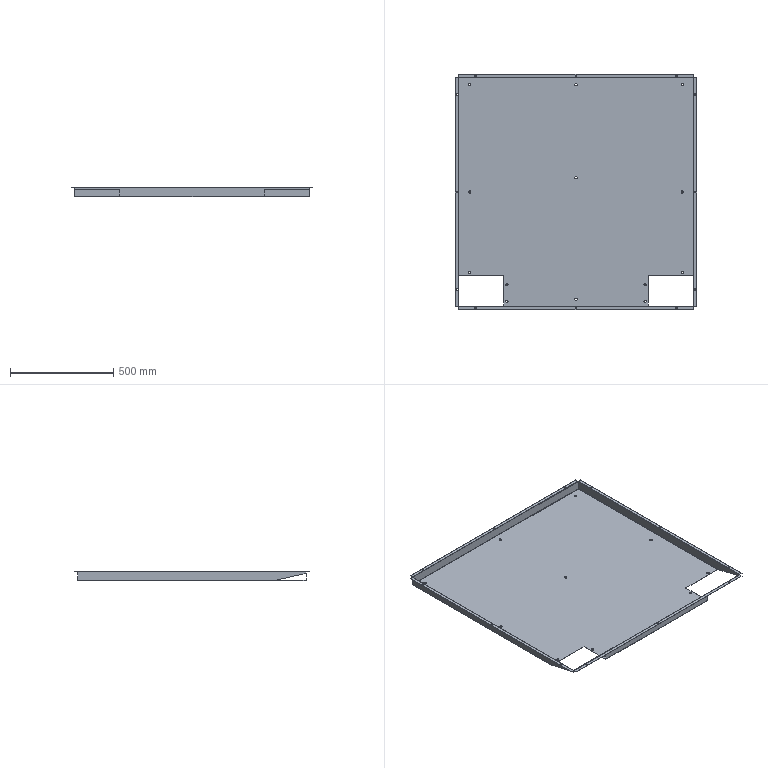Part | 1 solid | 160 faces | box 1170 x 1140 x 45 mm | volume 1439478 mm3 | plane 84 | cylinder 72 | spline 4 | commonest cylinder face diameters 7 x30 11 x26 0.4 x8 2.4 x8